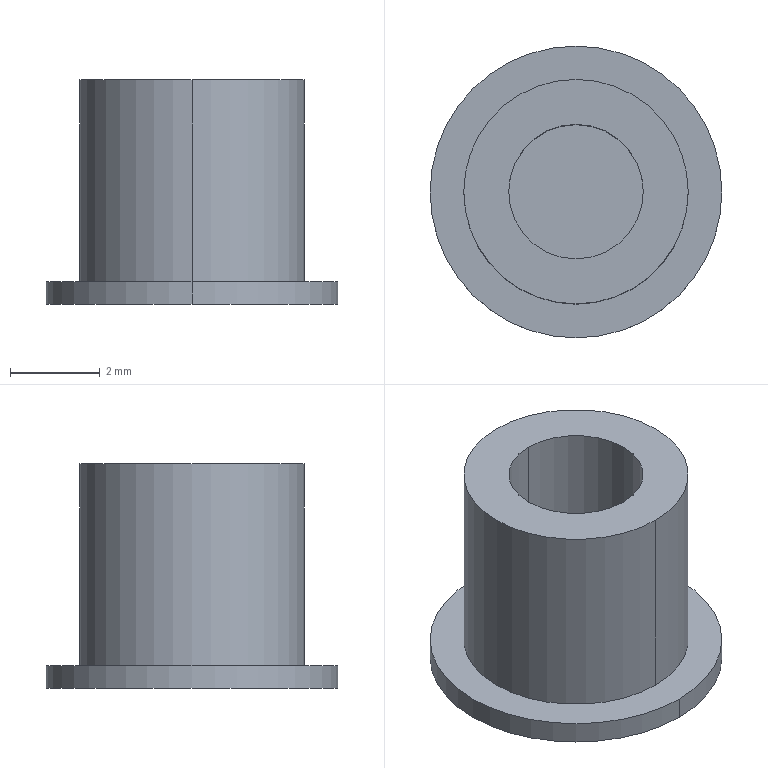Part | STEP file | LRS-150-12_X2_5F00517375-151323 | 1 solid | 10 faces | box 6.5 x 6.5 x 5 mm | volume 70.313 mm3 | cylinder 6 | plane 4 | commonest cylinder face diameters 3 x2 5 x2 6.5 x2
STEP:
#1=CARTESIAN_POINT('',(0.,0.,0.));
#2=DIRECTION('',(0.,0.,1.));
#3=DIRECTION('',(1.,0.,0.));
#4=AXIS2_PLACEMENT_3D('',#1,#2,#3);
#5=CARTESIAN_POINT('',(-271.167,266.625,-6.7));
#6=VERTEX_POINT('',#5);
#7=CARTESIAN_POINT('',(-271.167,263.625,-6.7));
#8=VERTEX_POINT('',#7);
#9=CARTESIAN_POINT('',(-271.167,265.125,-6.7));
#10=DIRECTION('',(0.,0.,1.));
#11=DIRECTION('',(0.,1.,0.));
#12=AXIS2_PLACEMENT_3D('',#9,#10,#11);
#13=CIRCLE('',#12,1.5);
#14=CARTESIAN_POINT('',(-271.167,264.375,-6.7));
#15=DIRECTION('',(0.,0.,-1.));
#16=DIRECTION('',(0.,1.,0.));
#17=AXIS2_PLACEMENT_3D('',#14,#15,#16);
#18=PLANE('',#17);
#19=CARTESIAN_POINT('',(2.25,0.));
#20=CARTESIAN_POINT('',(2.25,-2.598));
#21=CARTESIAN_POINT('',(0.,-1.299));
#22=CARTESIAN_POINT('',(-2.25,0.));
#23=CARTESIAN_POINT('',(0.,1.299));
#24=CARTESIAN_POINT('',(2.25,2.598));
#25=CARTESIAN_POINT('',(2.25,0.));
#26=(BOUNDED_CURVE()B_SPLINE_CURVE(2,(#19,#20,#21,#22,#23,#24,#25),.UNSPECIFIED.,.T.,.F.)B_SPLINE_CURVE_WITH_KNOTS((1,2,2,2,2,1),(-2.094,0.,2.094,4.189,6.283,8.378),.UNSPECIFIED.)CURVE()GEOMETRIC_REPRESENTATION_ITEM()RATIONAL_B_SPLINE_CURVE((1.,0.5,1.,0.5,1.,0.5,1.))REPRESENTATION_ITEM(''));
#27=(GEOMETRIC_REPRESENTATION_CONTEXT(2)PARAMETRIC_REPRESENTATION_CONTEXT()REPRESENTATION_CONTEXT('',''));
#28=DEFINITIONAL_REPRESENTATION('',(#26),#27);
#29=PCURVE('',#18,#28);
#30=CARTESIAN_POINT('',(-271.167,265.125,-1.6));
#31=DIRECTION('',(0.,0.,-1.));
#32=DIRECTION('',(0.,1.,0.));
#33=AXIS2_PLACEMENT_3D('',#30,#31,#32);
#34=CYLINDRICAL_SURFACE('',#33,1.5);
#35=CARTESIAN_POINT('',(6.283,5.1));
#36=DIRECTION('',(-1.,0.));
#37=VECTOR('',#36,1.);
#38=LINE('',#35,#37);
#39=(GEOMETRIC_REPRESENTATION_CONTEXT(2)PARAMETRIC_REPRESENTATION_CONTEXT()REPRESENTATION_CONTEXT('',''));
#40=DEFINITIONAL_REPRESENTATION('',(#38),#39);
#41=PCURVE('',#34,#40);
#42=SURFACE_CURVE('',#13,(#29,#41),.PCURVE_S1.);
#43=EDGE_CURVE('',#6,#8,#42,.T.);
#44=ORIENTED_EDGE('',*,*,#43,.F.);
#45=CARTESIAN_POINT('',(-271.167,265.125,-6.7));
#46=DIRECTION('',(0.,0.,1.));
#47=DIRECTION('',(0.,-1.,0.));
#48=AXIS2_PLACEMENT_3D('',#45,#46,#47);
#49=CIRCLE('',#48,1.5);
#50=CARTESIAN_POINT('',(-0.75,0.));
#51=CARTESIAN_POINT('',(-0.75,2.598));
#52=CARTESIAN_POINT('',(1.5,1.299));
#53=CARTESIAN_POINT('',(3.75,0.));
#54=CARTESIAN_POINT('',(1.5,-1.299));
#55=CARTESIAN_POINT('',(-0.75,-2.598));
#56=CARTESIAN_POINT('',(-0.75,0.));
#57=(BOUNDED_CURVE()B_SPLINE_CURVE(2,(#50,#51,#52,#53,#54,#55,#56),.UNSPECIFIED.,.T.,.F.)B_SPLINE_CURVE_WITH_KNOTS((1,2,2,2,2,1),(-2.094,0.,2.094,4.189,6.283,8.378),.UNSPECIFIED.)CURVE()GEOMETRIC_REPRESENTATION_ITEM()RATIONAL_B_SPLINE_CURVE((1.,0.5,1.,0.5,1.,0.5,1.))REPRESENTATION_ITEM(''));
#58=(GEOMETRIC_REPRESENTATION_CONTEXT(2)PARAMETRIC_REPRESENTATION_CONTEXT()REPRESENTATION_CONTEXT('',''));
#59=DEFINITIONAL_REPRESENTATION('',(#57),#58);
#60=PCURVE('',#18,#59);
#61=CARTESIAN_POINT('',(-271.167,265.125,-1.6));
#62=DIRECTION('',(0.,0.,-1.));
#63=DIRECTION('',(0.,1.,0.));
#64=AXIS2_PLACEMENT_3D('',#61,#62,#63);
#65=CYLINDRICAL_SURFACE('',#64,1.5);
#66=CARTESIAN_POINT('',(3.142,5.1));
#67=DIRECTION('',(-1.,0.));
#68=VECTOR('',#67,1.);
#69=LINE('',#66,#68);
#70=(GEOMETRIC_REPRESENTATION_CONTEXT(2)PARAMETRIC_REPRESENTATION_CONTEXT()REPRESENTATION_CONTEXT('',''));
#71=DEFINITIONAL_REPRESENTATION('',(#69),#70);
#72=PCURVE('',#65,#71);
#73=SURFACE_CURVE('',#49,(#60,#72),.PCURVE_S1.);
#74=EDGE_CURVE('',#8,#6,#73,.T.);
#75=ORIENTED_EDGE('',*,*,#74,.F.);
#76=EDGE_LOOP('',(#44,#75));
#77=FACE_BOUND('',#76,.F.);
#78=ADVANCED_FACE('',(#77),#18,.F.);
#79=CARTESIAN_POINT('',(-271.167,263.625,-1.8));
#80=VERTEX_POINT('',#79);
#81=CARTESIAN_POINT('',(-271.167,266.625,-1.8));
#82=VERTEX_POINT('',#81);
#83=CARTESIAN_POINT('',(-271.167,265.125,-1.8));
#84=DIRECTION('',(0.,0.,-1.));
#85=DIRECTION('',(0.,-1.,0.));
#86=AXIS2_PLACEMENT_3D('',#83,#84,#85);
#87=CIRCLE('',#86,1.5);
#88=CARTESIAN_POINT('',(3.142,0.2));
#89=DIRECTION('',(1.,0.));
#90=VECTOR('',#89,1.);
#91=LINE('',#88,#90);
#92=(GEOMETRIC_REPRESENTATION_CONTEXT(2)PARAMETRIC_REPRESENTATION_CONTEXT()REPRESENTATION_CONTEXT('',''));
#93=DEFINITIONAL_REPRESENTATION('',(#91),#92);
#94=PCURVE('',#34,#93);
#95=CARTESIAN_POINT('',(-271.167,263.125,-1.8));
#96=DIRECTION('',(0.,0.,-1.));
#97=DIRECTION('',(0.,1.,0.));
#98=AXIS2_PLACEMENT_3D('',#95,#96,#97);
#99=PLANE('',#98);
#100=CARTESIAN_POINT('',(2.,0.));
#101=DIRECTION('',(-1.,0.));
#102=AXIS2_PLACEMENT_2D('',#100,#101);
#103=CIRCLE('',#102,1.5);
#104=(GEOMETRIC_REPRESENTATION_CONTEXT(2)PARAMETRIC_REPRESENTATION_CONTEXT()REPRESENTATION_CONTEXT('',''));
#105=DEFINITIONAL_REPRESENTATION('',(#103),#104);
#106=PCURVE('',#99,#105);
#107=SURFACE_CURVE('',#87,(#94,#106),.PCURVE_S1.);
#108=EDGE_CURVE('',#80,#82,#107,.T.);
#109=ORIENTED_EDGE('',*,*,#108,.T.);
#110=CARTESIAN_POINT('',(-271.167,266.625,-6.7));
#111=DIRECTION('',(0.,0.,1.));
#112=VECTOR('',#111,1.);
#113=LINE('',#110,#112);
#114=CARTESIAN_POINT('',(6.283,5.1));
#115=DIRECTION('',(0.,-1.));
#116=VECTOR('',#115,1.);
#117=LINE('',#114,#116);
#118=(GEOMETRIC_REPRESENTATION_CONTEXT(2)PARAMETRIC_REPRESENTATION_CONTEXT()REPRESENTATION_CONTEXT('',''));
#119=DEFINITIONAL_REPRESENTATION('',(#117),#118);
#120=PCURVE('',#34,#119);
#121=CARTESIAN_POINT('',(0.,5.1));
#122=DIRECTION('',(0.,-1.));
#123=VECTOR('',#122,1.);
#124=LINE('',#121,#123);
#125=(GEOMETRIC_REPRESENTATION_CONTEXT(2)PARAMETRIC_REPRESENTATION_CONTEXT()REPRESENTATION_CONTEXT('',''));
#126=DEFINITIONAL_REPRESENTATION('',(#124),#125);
#127=PCURVE('',#65,#126);
#128=SURFACE_CURVE('',#113,(#120,#127),.PCURVE_S1.);
#129=EDGE_CURVE('',#6,#82,#128,.T.);
#130=ORIENTED_EDGE('',*,*,#129,.F.);
#131=ORIENTED_EDGE('',*,*,#43,.T.);
#132=CARTESIAN_POINT('',(-271.167,263.625,-6.7));
#133=DIRECTION('',(0.,0.,1.));
#134=VECTOR('',#133,1.);
#135=LINE('',#132,#134);
#136=CARTESIAN_POINT('',(3.142,5.1));
#137=DIRECTION('',(0.,-1.));
#138=VECTOR('',#137,1.);
#139=LINE('',#136,#138);
#140=(GEOMETRIC_REPRESENTATION_CONTEXT(2)PARAMETRIC_REPRESENTATION_CONTEXT()REPRESENTATION_CONTEXT('',''));
#141=DEFINITIONAL_REPRESENTATION('',(#139),#140);
#142=PCURVE('',#34,#141);
#143=CARTESIAN_POINT('',(3.142,5.1));
#144=DIRECTION('',(0.,-1.));
#145=VECTOR('',#144,1.);
#146=LINE('',#143,#145);
#147=(GEOMETRIC_REPRESENTATION_CONTEXT(2)PARAMETRIC_REPRESENTATION_CONTEXT()REPRESENTATION_CONTEXT('',''));
#148=DEFINITIONAL_REPRESENTATION('',(#146),#147);
#149=PCURVE('',#65,#148);
#150=SURFACE_CURVE('',#135,(#142,#149),.PCURVE_S1.);
#151=EDGE_CURVE('',#8,#80,#150,.T.);
#152=ORIENTED_EDGE('',*,*,#151,.T.);
#153=EDGE_LOOP('',(#109,#130,#131,#152));
#154=FACE_BOUND('',#153,.F.);
#155=ADVANCED_FACE('',(#154),#34,.F.);
#156=CARTESIAN_POINT('',(-271.167,267.625,-1.8));
#157=VERTEX_POINT('',#156);
#158=CARTESIAN_POINT('',(-271.167,262.625,-1.8));
#159=VERTEX_POINT('',#158);
#160=CARTESIAN_POINT('',(-271.167,265.125,-1.8));
#161=DIRECTION('',(0.,0.,1.));
#162=DIRECTION('',(0.,1.,0.));
#163=AXIS2_PLACEMENT_3D('',#160,#161,#162);
#164=CIRCLE('',#163,2.5);
#165=CARTESIAN_POINT('',(4.5,0.));
#166=CARTESIAN_POINT('',(4.5,-4.33));
#167=CARTESIAN_POINT('',(0.75,-2.165));
#168=CARTESIAN_POINT('',(-3.,0.));
#169=CARTESIAN_POINT('',(0.75,2.165));
#170=CARTESIAN_POINT('',(4.5,4.33));
#171=CARTESIAN_POINT('',(4.5,0.));
#172=(BOUNDED_CURVE()B_SPLINE_CURVE(2,(#165,#166,#167,#168,#169,#170,#171),.UNSPECIFIED.,.T.,.F.)B_SPLINE_CURVE_WITH_KNOTS((1,2,2,2,2,1),(-2.094,0.,2.094,4.189,6.283,8.378),.UNSPECIFIED.)CURVE()GEOMETRIC_REPRESENTATION_ITEM()RATIONAL_B_SPLINE_CURVE((1.,0.5,1.,0.5,1.,0.5,1.))REPRESENTATION_ITEM(''));
#173=(GEOMETRIC_REPRESENTATION_CONTEXT(2)PARAMETRIC_REPRESENTATION_CONTEXT()REPRESENTATION_CONTEXT('',''));
#174=DEFINITIONAL_REPRESENTATION('',(#172),#173);
#175=PCURVE('',#99,#174);
#176=CARTESIAN_POINT('',(-271.167,265.125,-2.3));
#177=DIRECTION('',(0.,0.,-1.));
#178=DIRECTION('',(0.,1.,0.));
#179=AXIS2_PLACEMENT_3D('',#176,#177,#178);
#180=CYLINDRICAL_SURFACE('',#179,2.5);
#181=CARTESIAN_POINT('',(6.283,-0.5));
#182=DIRECTION('',(-1.,0.));
#183=VECTOR('',#182,1.);
#184=LINE('',#181,#183);
#185=(GEOMETRIC_REPRESENTATION_CONTEXT(2)PARAMETRIC_REPRESENTATION_CONTEXT()REPRESENTATION_CONTEXT('',''));
#186=DEFINITIONAL_REPRESENTATION('',(#184),#185);
#187=PCURVE('',#180,#186);
#188=SURFACE_CURVE('',#164,(#175,#187),.PCURVE_S1.);
#189=EDGE_CURVE('',#157,#159,#188,.T.);
#190=ORIENTED_EDGE('',*,*,#189,.F.);
#191=CARTESIAN_POINT('',(-271.167,265.125,-1.8));
#192=DIRECTION('',(0.,0.,1.));
#193=DIRECTION('',(0.,-1.,0.));
#194=AXIS2_PLACEMENT_3D('',#191,#192,#193);
#195=CIRCLE('',#194,2.5);
#196=CARTESIAN_POINT('',(-0.5,0.));
#197=CARTESIAN_POINT('',(-0.5,4.33));
#198=CARTESIAN_POINT('',(3.25,2.165));
#199=CARTESIAN_POINT('',(7.,0.));
#200=CARTESIAN_POINT('',(3.25,-2.165));
#201=CARTESIAN_POINT('',(-0.5,-4.33));
#202=CARTESIAN_POINT('',(-0.5,0.));
#203=(BOUNDED_CURVE()B_SPLINE_CURVE(2,(#196,#197,#198,#199,#200,#201,#202),.UNSPECIFIED.,.T.,.F.)B_SPLINE_CURVE_WITH_KNOTS((1,2,2,2,2,1),(-2.094,0.,2.094,4.189,6.283,8.378),.UNSPECIFIED.)CURVE()GEOMETRIC_REPRESENTATION_ITEM()RATIONAL_B_SPLINE_CURVE((1.,0.5,1.,0.5,1.,0.5,1.))REPRESENTATION_ITEM(''));
#204=(GEOMETRIC_REPRESENTATION_CONTEXT(2)PARAMETRIC_REPRESENTATION_CONTEXT()REPRESENTATION_CONTEXT('',''));
#205=DEFINITIONAL_REPRESENTATION('',(#203),#204);
#206=PCURVE('',#99,#205);
#207=CARTESIAN_POINT('',(-271.167,265.125,-2.3));
#208=DIRECTION('',(0.,0.,-1.));
#209=DIRECTION('',(0.,1.,0.));
#210=AXIS2_PLACEMENT_3D('',#207,#208,#209);
#211=CYLINDRICAL_SURFACE('',#210,2.5);
#212=CARTESIAN_POINT('',(3.142,-0.5));
#213=DIRECTION('',(-1.,0.));
#214=VECTOR('',#213,1.);
#215=LINE('',#212,#214);
#216=(GEOMETRIC_REPRESENTATION_CONTEXT(2)PARAMETRIC_REPRESENTATION_CONTEXT()REPRESENTATION_CONTEXT('',''));
#217=DEFINITIONAL_REPRESENTATION('',(#215),#216);
#218=PCURVE('',#211,#217);
#219=SURFACE_CURVE('',#195,(#206,#218),.PCURVE_S1.);
#220=EDGE_CURVE('',#159,#157,#219,.T.);
#221=ORIENTED_EDGE('',*,*,#220,.F.);
#222=EDGE_LOOP('',(#190,#221));
#223=FACE_BOUND('',#222,.F.);
#224=ORIENTED_EDGE('',*,*,#108,.F.);
#225=CARTESIAN_POINT('',(-271.167,265.125,-1.8));
#226=DIRECTION('',(0.,0.,-1.));
#227=DIRECTION('',(0.,1.,0.));
#228=AXIS2_PLACEMENT_3D('',#225,#226,#227);
#229=CIRCLE('',#228,1.5);
#230=CARTESIAN_POINT('',(2.,0.));
#231=DIRECTION('',(1.,0.));
#232=AXIS2_PLACEMENT_2D('',#230,#231);
#233=CIRCLE('',#232,1.5);
#234=(GEOMETRIC_REPRESENTATION_CONTEXT(2)PARAMETRIC_REPRESENTATION_CONTEXT()REPRESENTATION_CONTEXT('',''));
#235=DEFINITIONAL_REPRESENTATION('',(#233),#234);
#236=PCURVE('',#99,#235);
#237=CARTESIAN_POINT('',(0.,0.2));
#238=DIRECTION('',(1.,0.));
#239=VECTOR('',#238,1.);
#240=LINE('',#237,#239);
#241=(GEOMETRIC_REPRESENTATION_CONTEXT(2)PARAMETRIC_REPRESENTATION_CONTEXT()REPRESENTATION_CONTEXT('',''));
#242=DEFINITIONAL_REPRESENTATION('',(#240),#241);
#243=PCURVE('',#65,#242);
#244=SURFACE_CURVE('',#229,(#236,#243),.PCURVE_S1.);
#245=EDGE_CURVE('',#82,#80,#244,.T.);
#246=ORIENTED_EDGE('',*,*,#245,.F.);
#247=EDGE_LOOP('',(#224,#246));
#248=FACE_BOUND('',#247,.F.);
#249=ADVANCED_FACE('',(#223,#248),#99,.F.);
#250=ORIENTED_EDGE('',*,*,#245,.T.);
#251=ORIENTED_EDGE('',*,*,#151,.F.);
#252=ORIENTED_EDGE('',*,*,#74,.T.);
#253=ORIENTED_EDGE('',*,*,#129,.T.);
#254=EDGE_LOOP('',(#250,#251,#252,#253));
#255=FACE_BOUND('',#254,.F.);
#256=ADVANCED_FACE('',(#255),#65,.F.);
#257=CARTESIAN_POINT('',(-271.167,267.625,-6.3));
#258=VERTEX_POINT('',#257);
#259=CARTESIAN_POINT('',(-271.167,267.625,-1.8));
#260=DIRECTION('',(0.,0.,-1.));
#261=VECTOR('',#260,1.);
#262=LINE('',#259,#261);
#263=CARTESIAN_POINT('',(6.283,-0.5));
#264=DIRECTION('',(0.,1.));
#265=VECTOR('',#264,1.);
#266=LINE('',#263,#265);
#267=(GEOMETRIC_REPRESENTATION_CONTEXT(2)PARAMETRIC_REPRESENTATION_CONTEXT()REPRESENTATION_CONTEXT('',''));
#268=DEFINITIONAL_REPRESENTATION('',(#266),#267);
#269=PCURVE('',#180,#268);
#270=CARTESIAN_POINT('',(0.,-0.5));
#271=DIRECTION('',(0.,1.));
#272=VECTOR('',#271,1.);
#273=LINE('',#270,#272);
#274=(GEOMETRIC_REPRESENTATION_CONTEXT(2)PARAMETRIC_REPRESENTATION_CONTEXT()REPRESENTATION_CONTEXT('',''));
#275=DEFINITIONAL_REPRESENTATION('',(#273),#274);
#276=PCURVE('',#211,#275);
#277=SURFACE_CURVE('',#262,(#269,#276),.PCURVE_S1.);
#278=EDGE_CURVE('',#157,#258,#277,.T.);
#279=ORIENTED_EDGE('',*,*,#278,.T.);
#280=CARTESIAN_POINT('',(-271.167,262.625,-6.3));
#281=VERTEX_POINT('',#280);
#282=CARTESIAN_POINT('',(-271.167,265.125,-6.3));
#283=DIRECTION('',(0.,0.,-1.));
#284=DIRECTION('',(0.,-1.,0.));
#285=AXIS2_PLACEMENT_3D('',#282,#283,#284);
#286=CIRCLE('',#285,2.5);
#287=CARTESIAN_POINT('',(3.142,4.));
#288=DIRECTION('',(1.,0.));
#289=VECTOR('',#288,1.);
#290=LINE('',#287,#289);
#291=(GEOMETRIC_REPRESENTATION_CONTEXT(2)PARAMETRIC_REPRESENTATION_CONTEXT()REPRESENTATION_CONTEXT('',''));
#292=DEFINITIONAL_REPRESENTATION('',(#290),#291);
#293=PCURVE('',#180,#292);
#294=CARTESIAN_POINT('',(-271.167,262.125,-6.3));
#295=DIRECTION('',(0.,0.,-1.));
#296=DIRECTION('',(0.,1.,0.));
#297=AXIS2_PLACEMENT_3D('',#294,#295,#296);
#298=PLANE('',#297);
#299=CARTESIAN_POINT('',(3.,0.));
#300=DIRECTION('',(-1.,0.));
#301=AXIS2_PLACEMENT_2D('',#299,#300);
#302=CIRCLE('',#301,2.5);
#303=(GEOMETRIC_REPRESENTATION_CONTEXT(2)PARAMETRIC_REPRESENTATION_CONTEXT()REPRESENTATION_CONTEXT('',''));
#304=DEFINITIONAL_REPRESENTATION('',(#302),#303);
#305=PCURVE('',#298,#304);
#306=SURFACE_CURVE('',#286,(#293,#305),.PCURVE_S1.);
#307=EDGE_CURVE('',#281,#258,#306,.T.);
#308=ORIENTED_EDGE('',*,*,#307,.F.);
#309=CARTESIAN_POINT('',(-271.167,262.625,-1.8));
#310=DIRECTION('',(0.,0.,-1.));
#311=VECTOR('',#310,1.);
#312=LINE('',#309,#311);
#313=CARTESIAN_POINT('',(3.142,-0.5));
#314=DIRECTION('',(0.,1.));
#315=VECTOR('',#314,1.);
#316=LINE('',#313,#315);
#317=(GEOMETRIC_REPRESENTATION_CONTEXT(2)PARAMETRIC_REPRESENTATION_CONTEXT()REPRESENTATION_CONTEXT('',''));
#318=DEFINITIONAL_REPRESENTATION('',(#316),#317);
#319=PCURVE('',#180,#318);
#320=CARTESIAN_POINT('',(3.142,-0.5));
#321=DIRECTION('',(0.,1.));
#322=VECTOR('',#321,1.);
#323=LINE('',#320,#322);
#324=(GEOMETRIC_REPRESENTATION_CONTEXT(2)PARAMETRIC_REPRESENTATION_CONTEXT()REPRESENTATION_CONTEXT('',''));
#325=DEFINITIONAL_REPRESENTATION('',(#323),#324);
#326=PCURVE('',#211,#325);
#327=SURFACE_CURVE('',#312,(#319,#326),.PCURVE_S1.);
#328=EDGE_CURVE('',#159,#281,#327,.T.);
#329=ORIENTED_EDGE('',*,*,#328,.F.);
#330=ORIENTED_EDGE('',*,*,#189,.F.);
#331=EDGE_LOOP('',(#279,#308,#329,#330));
#332=FACE_BOUND('',#331,.T.);
#333=ADVANCED_FACE('',(#332),#180,.T.);
#334=CARTESIAN_POINT('',(-271.167,265.125,-6.3));
#335=DIRECTION('',(0.,0.,-1.));
#336=DIRECTION('',(0.,1.,0.));
#337=AXIS2_PLACEMENT_3D('',#334,#335,#336);
#338=CIRCLE('',#337,2.5);
#339=CARTESIAN_POINT('',(0.,4.));
#340=DIRECTION('',(1.,0.));
#341=VECTOR('',#340,1.);
#342=LINE('',#339,#341);
#343=(GEOMETRIC_REPRESENTATION_CONTEXT(2)PARAMETRIC_REPRESENTATION_CONTEXT()REPRESENTATION_CONTEXT('',''));
#344=DEFINITIONAL_REPRESENTATION('',(#342),#343);
#345=PCURVE('',#211,#344);
#346=CARTESIAN_POINT('',(3.,0.));
#347=DIRECTION('',(1.,0.));
#348=AXIS2_PLACEMENT_2D('',#346,#347);
#349=CIRCLE('',#348,2.5);
#350=(GEOMETRIC_REPRESENTATION_CONTEXT(2)PARAMETRIC_REPRESENTATION_CONTEXT()REPRESENTATION_CONTEXT('',''));
#351=DEFINITIONAL_REPRESENTATION('',(#349),#350);
#352=PCURVE('',#298,#351);
#353=SURFACE_CURVE('',#338,(#345,#352),.PCURVE_S1.);
#354=EDGE_CURVE('',#258,#281,#353,.T.);
#355=ORIENTED_EDGE('',*,*,#354,.F.);
#356=ORIENTED_EDGE('',*,*,#278,.F.);
#357=ORIENTED_EDGE('',*,*,#220,.F.);
#358=ORIENTED_EDGE('',*,*,#328,.T.);
#359=EDGE_LOOP('',(#355,#356,#357,#358));
#360=FACE_BOUND('',#359,.T.);
#361=ADVANCED_FACE('',(#360),#211,.T.);
#362=CARTESIAN_POINT('',(-271.167,268.375,-6.3));
#363=VERTEX_POINT('',#362);
#364=CARTESIAN_POINT('',(-271.167,261.875,-6.3));
#365=VERTEX_POINT('',#364);
#366=CARTESIAN_POINT('',(-271.167,265.125,-6.3));
#367=DIRECTION('',(0.,0.,1.));
#368=DIRECTION('',(0.,1.,0.));
#369=AXIS2_PLACEMENT_3D('',#366,#367,#368);
#370=CIRCLE('',#369,3.25);
#371=CARTESIAN_POINT('',(6.25,0.));
#372=CARTESIAN_POINT('',(6.25,-5.629));
#373=CARTESIAN_POINT('',(1.375,-2.815));
#374=CARTESIAN_POINT('',(-3.5,0.));
#375=CARTESIAN_POINT('',(1.375,2.815));
#376=CARTESIAN_POINT('',(6.25,5.629));
#377=CARTESIAN_POINT('',(6.25,0.));
#378=(BOUNDED_CURVE()B_SPLINE_CURVE(2,(#371,#372,#373,#374,#375,#376,#377),.UNSPECIFIED.,.T.,.F.)B_SPLINE_CURVE_WITH_KNOTS((1,2,2,2,2,1),(-2.094,0.,2.094,4.189,6.283,8.378),.UNSPECIFIED.)CURVE()GEOMETRIC_REPRESENTATION_ITEM()RATIONAL_B_SPLINE_CURVE((1.,0.5,1.,0.5,1.,0.5,1.))REPRESENTATION_ITEM(''));
#379=(GEOMETRIC_REPRESENTATION_CONTEXT(2)PARAMETRIC_REPRESENTATION_CONTEXT()REPRESENTATION_CONTEXT('',''));
#380=DEFINITIONAL_REPRESENTATION('',(#378),#379);
#381=PCURVE('',#298,#380);
#382=CARTESIAN_POINT('',(-271.167,265.125,-7.3));
#383=DIRECTION('',(0.,0.,-1.));
#384=DIRECTION('',(0.,1.,0.));
#385=AXIS2_PLACEMENT_3D('',#382,#383,#384);
#386=CYLINDRICAL_SURFACE('',#385,3.25);
#387=CARTESIAN_POINT('',(6.283,-1.));
#388=DIRECTION('',(-1.,0.));
#389=VECTOR('',#388,1.);
#390=LINE('',#387,#389);
#391=(GEOMETRIC_REPRESENTATION_CONTEXT(2)PARAMETRIC_REPRESENTATION_CONTEXT()REPRESENTATION_CONTEXT('',''));
#392=DEFINITIONAL_REPRESENTATION('',(#390),#391);
#393=PCURVE('',#386,#392);
#394=SURFACE_CURVE('',#370,(#381,#393),.PCURVE_S1.);
#395=EDGE_CURVE('',#363,#365,#394,.T.);
#396=ORIENTED_EDGE('',*,*,#395,.F.);
#397=CARTESIAN_POINT('',(-271.167,265.125,-6.3));
#398=DIRECTION('',(0.,0.,1.));
#399=DIRECTION('',(0.,-1.,0.));
#400=AXIS2_PLACEMENT_3D('',#397,#398,#399);
#401=CIRCLE('',#400,3.25);
#402=CARTESIAN_POINT('',(-0.25,0.));
#403=CARTESIAN_POINT('',(-0.25,5.629));
#404=CARTESIAN_POINT('',(4.625,2.815));
#405=CARTESIAN_POINT('',(9.5,0.));
#406=CARTESIAN_POINT('',(4.625,-2.815));
#407=CARTESIAN_POINT('',(-0.25,-5.629));
#408=CARTESIAN_POINT('',(-0.25,0.));
#409=(BOUNDED_CURVE()B_SPLINE_CURVE(2,(#402,#403,#404,#405,#406,#407,#408),.UNSPECIFIED.,.T.,.F.)B_SPLINE_CURVE_WITH_KNOTS((1,2,2,2,2,1),(-2.094,0.,2.094,4.189,6.283,8.378),.UNSPECIFIED.)CURVE()GEOMETRIC_REPRESENTATION_ITEM()RATIONAL_B_SPLINE_CURVE((1.,0.5,1.,0.5,1.,0.5,1.))REPRESENTATION_ITEM(''));
#410=(GEOMETRIC_REPRESENTATION_CONTEXT(2)PARAMETRIC_REPRESENTATION_CONTEXT()REPRESENTATION_CONTEXT('',''));
#411=DEFINITIONAL_REPRESENTATION('',(#409),#410);
#412=PCURVE('',#298,#411);
#413=CARTESIAN_POINT('',(-271.167,265.125,-7.3));
#414=DIRECTION('',(0.,0.,-1.));
#415=DIRECTION('',(0.,1.,0.));
#416=AXIS2_PLACEMENT_3D('',#413,#414,#415);
#417=CYLINDRICAL_SURFACE('',#416,3.25);
#418=CARTESIAN_POINT('',(3.142,-1.));
#419=DIRECTION('',(-1.,0.));
#420=VECTOR('',#419,1.);
#421=LINE('',#418,#420);
#422=(GEOMETRIC_REPRESENTATION_CONTEXT(2)PARAMETRIC_REPRESENTATION_CONTEXT()REPRESENTATION_CONTEXT('',''));
#423=DEFINITIONAL_REPRESENTATION('',(#421),#422);
#424=PCURVE('',#417,#423);
#425=SURFACE_CURVE('',#401,(#412,#424),.PCURVE_S1.);
#426=EDGE_CURVE('',#365,#363,#425,.T.);
#427=ORIENTED_EDGE('',*,*,#426,.F.);
#428=EDGE_LOOP('',(#396,#427));
#429=FACE_BOUND('',#428,.F.);
#430=ORIENTED_EDGE('',*,*,#307,.F.);
#431=ORIENTED_EDGE('',*,*,#354,.F.);
#432=EDGE_LOOP('',(#430,#431));
#433=FACE_BOUND('',#432,.F.);
#434=ADVANCED_FACE('',(#429,#433),#298,.F.);
#435=CARTESIAN_POINT('',(-271.167,268.375,-6.8));
#436=VERTEX_POINT('',#435);
#437=CARTESIAN_POINT('',(-271.167,268.375,-6.3));
#438=DIRECTION('',(0.,0.,-1.));
#439=VECTOR('',#438,1.);
#440=LINE('',#437,#439);
#441=CARTESIAN_POINT('',(6.283,-1.));
#442=DIRECTION('',(0.,1.));
#443=VECTOR('',#442,1.);
#444=LINE('',#441,#443);
#445=(GEOMETRIC_REPRESENTATION_CONTEXT(2)PARAMETRIC_REPRESENTATION_CONTEXT()REPRESENTATION_CONTEXT('',''));
#446=DEFINITIONAL_REPRESENTATION('',(#444),#445);
#447=PCURVE('',#386,#446);
#448=CARTESIAN_POINT('',(0.,-1.));
#449=DIRECTION('',(0.,1.));
#450=VECTOR('',#449,1.);
#451=LINE('',#448,#450);
#452=(GEOMETRIC_REPRESENTATION_CONTEXT(2)PARAMETRIC_REPRESENTATION_CONTEXT()REPRESENTATION_CONTEXT('',''));
#453=DEFINITIONAL_REPRESENTATION('',(#451),#452);
#454=PCURVE('',#417,#453);
#455=SURFACE_CURVE('',#440,(#447,#454),.PCURVE_S1.);
#456=EDGE_CURVE('',#363,#436,#455,.T.);
#457=ORIENTED_EDGE('',*,*,#456,.T.);
#458=CARTESIAN_POINT('',(-271.167,261.875,-6.8));
#459=VERTEX_POINT('',#458);
#460=CARTESIAN_POINT('',(-271.167,265.125,-6.8));
#461=DIRECTION('',(0.,0.,-1.));
#462=DIRECTION('',(0.,-1.,0.));
#463=AXIS2_PLACEMENT_3D('',#460,#461,#462);
#464=CIRCLE('',#463,3.25);
#465=CARTESIAN_POINT('',(3.142,-0.5));
#466=DIRECTION('',(1.,0.));
#467=VECTOR('',#466,1.);
#468=LINE('',#465,#467);
#469=(GEOMETRIC_REPRESENTATION_CONTEXT(2)PARAMETRIC_REPRESENTATION_CONTEXT()REPRESENTATION_CONTEXT('',''));
#470=DEFINITIONAL_REPRESENTATION('',(#468),#469);
#471=PCURVE('',#386,#470);
#472=CARTESIAN_POINT('',(-502.167,272.595,-6.8));
#473=DIRECTION('',(0.,0.,-1.));
#474=DIRECTION('',(0.,-1.,0.));
#475=AXIS2_PLACEMENT_3D('',#472,#473,#474);
#476=PLANE('',#475);
#477=CARTESIAN_POINT('',(7.47,-231.));
#478=DIRECTION('',(1.,0.));
#479=AXIS2_PLACEMENT_2D('',#477,#478);
#480=CIRCLE('',#479,3.25);
#481=(GEOMETRIC_REPRESENTATION_CONTEXT(2)PARAMETRIC_REPRESENTATION_CONTEXT()REPRESENTATION_CONTEXT('',''));
#482=DEFINITIONAL_REPRESENTATION('',(#480),#481);
#483=PCURVE('',#476,#482);
#484=SURFACE_CURVE('',#464,(#471,#483),.PCURVE_S1.);
#485=EDGE_CURVE('',#459,#436,#484,.T.);
#486=ORIENTED_EDGE('',*,*,#485,.F.);
#487=CARTESIAN_POINT('',(-271.167,261.875,-6.3));
#488=DIRECTION('',(0.,0.,-1.));
#489=VECTOR('',#488,1.);
#490=LINE('',#487,#489);
#491=CARTESIAN_POINT('',(3.142,-1.));
#492=DIRECTION('',(0.,1.));
#493=VECTOR('',#492,1.);
#494=LINE('',#491,#493);
#495=(GEOMETRIC_REPRESENTATION_CONTEXT(2)PARAMETRIC_REPRESENTATION_CONTEXT()REPRESENTATION_CONTEXT('',''));
#496=DEFINITIONAL_REPRESENTATION('',(#494),#495);
#497=PCURVE('',#386,#496);
#498=CARTESIAN_POINT('',(3.142,-1.));
#499=DIRECTION('',(0.,1.));
#500=VECTOR('',#499,1.);
#501=LINE('',#498,#500);
#502=(GEOMETRIC_REPRESENTATION_CONTEXT(2)PARAMETRIC_REPRESENTATION_CONTEXT()REPRESENTATION_CONTEXT('',''));
#503=DEFINITIONAL_REPRESENTATION('',(#501),#502);
#504=PCURVE('',#417,#503);
#505=SURFACE_CURVE('',#490,(#497,#504),.PCURVE_S1.);
#506=EDGE_CURVE('',#365,#459,#505,.T.);
#507=ORIENTED_EDGE('',*,*,#506,.F.);
#508=ORIENTED_EDGE('',*,*,#395,.F.);
#509=EDGE_LOOP('',(#457,#486,#507,#508));
#510=FACE_BOUND('',#509,.T.);
#511=ADVANCED_FACE('',(#510),#386,.T.);
#512=CARTESIAN_POINT('',(-271.167,265.125,-6.8));
#513=DIRECTION('',(0.,0.,-1.));
#514=DIRECTION('',(0.,1.,0.));
#515=AXIS2_PLACEMENT_3D('',#512,#513,#514);
#516=CIRCLE('',#515,3.25);
#517=CARTESIAN_POINT('',(0.,-0.5));
#518=DIRECTION('',(1.,0.));
#519=VECTOR('',#518,1.);
#520=LINE('',#517,#519);
#521=(GEOMETRIC_REPRESENTATION_CONTEXT(2)PARAMETRIC_REPRESENTATION_CONTEXT()REPRESENTATION_CONTEXT('',''));
#522=DEFINITIONAL_REPRESENTATION('',(#520),#521);
#523=PCURVE('',#417,#522);
#524=CARTESIAN_POINT('',(7.47,-231.));
#525=DIRECTION('',(-1.,0.));
#526=AXIS2_PLACEMENT_2D('',#524,#525);
#527=CIRCLE('',#526,3.25);
#528=(GEOMETRIC_REPRESENTATION_CONTEXT(2)PARAMETRIC_REPRESENTATION_CONTEXT()REPRESENTATION_CONTEXT('',''));
#529=DEFINITIONAL_REPRESENTATION('',(#527),#528);
#530=PCURVE('',#476,#529);
#531=SURFACE_CURVE('',#516,(#523,#530),.PCURVE_S1.);
#532=EDGE_CURVE('',#436,#459,#531,.T.);
#533=ORIENTED_EDGE('',*,*,#532,.F.);
#534=ORIENTED_EDGE('',*,*,#456,.F.);
#535=ORIENTED_EDGE('',*,*,#426,.F.);
#536=ORIENTED_EDGE('',*,*,#506,.T.);
#537=EDGE_LOOP('',(#533,#534,#535,#536));
#538=FACE_BOUND('',#537,.T.);
#539=ADVANCED_FACE('',(#538),#417,.T.);
#540=ORIENTED_EDGE('',*,*,#485,.F.);
#541=ORIENTED_EDGE('',*,*,#532,.F.);
#542=EDGE_LOOP('',(#540,#541));
#543=FACE_BOUND('',#542,.F.);
#544=ADVANCED_FACE('',(#543),#476,.T.);
#545=CLOSED_SHELL('',(#78,#155,#249,#256,#333,#361,#434,#511,#539,#544));
#546=MANIFOLD_SOLID_BREP('',#545);
#547=(LENGTH_UNIT()NAMED_UNIT(*)SI_UNIT(.MILLI.,.METRE.));
#548=UNCERTAINTY_MEASURE_WITH_UNIT(LENGTH_MEASURE(0.0000001),#547,'','');
#549=(NAMED_UNIT(*)PLANE_ANGLE_UNIT()SI_UNIT($,.RADIAN.));
#550=(NAMED_UNIT(*)SI_UNIT($,.STERADIAN.)SOLID_ANGLE_UNIT());
#551=(GEOMETRIC_REPRESENTATION_CONTEXT(3)GLOBAL_UNCERTAINTY_ASSIGNED_CONTEXT((#548))GLOBAL_UNIT_ASSIGNED_CONTEXT((#547,#549,#550))REPRESENTATION_CONTEXT('',''));
#552=ADVANCED_BREP_SHAPE_REPRESENTATION('',(#4,#546),#551);